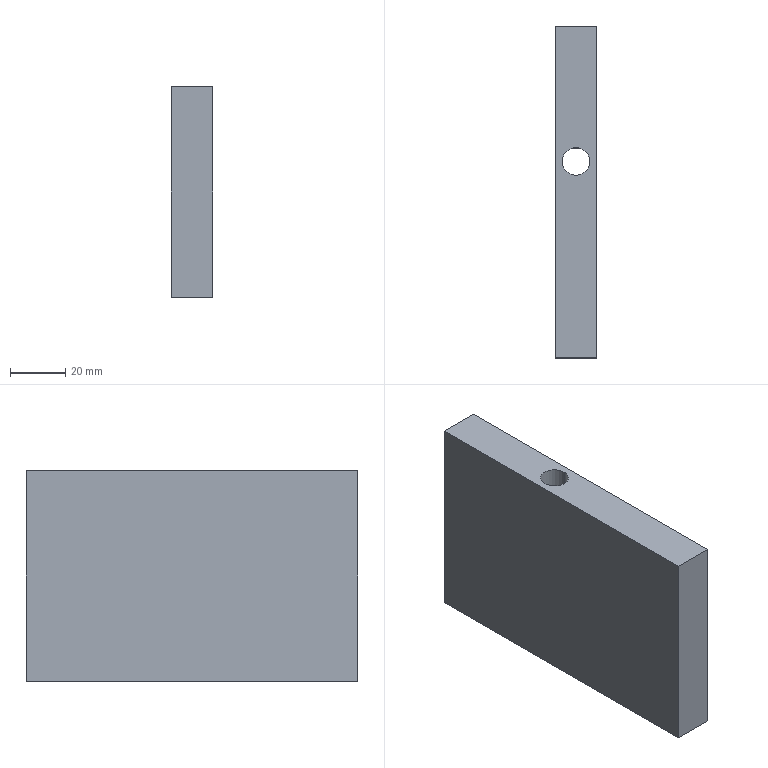Part | SolidWorks | features Extrusion 1, ICE 1 | 1 solid | 8 faces | box 15 x 120 x 76 mm | volume 130831 mm3 | plane 6 | cylinder 2 | commonest cylinder face diameters 10 x2
STEP:
#1=CARTESIAN_POINT('',(-5.,11.,0.));
#2=VERTEX_POINT('',#1);
#3=CARTESIAN_POINT('',(5.,11.,0.));
#4=VERTEX_POINT('',#3);
#5=CARTESIAN_POINT('',(0.,11.,0.));
#6=DIRECTION('',(0.,0.,1.));
#7=DIRECTION('',(1.,0.,0.));
#8=AXIS2_PLACEMENT_3D('',#5,#6,#7);
#9=CIRCLE('',#8,5.);
#10=EDGE_CURVE('',#2,#4,#9,.T.);
#11=ORIENTED_EDGE('',*,*,#10,.F.);
#12=CARTESIAN_POINT('',(-5.,11.,76.));
#13=VERTEX_POINT('',#12);
#14=CARTESIAN_POINT('',(-5.,11.,0.));
#15=DIRECTION('',(0.,0.,1.));
#16=VECTOR('',#15,1000.);
#17=LINE('',#14,#16);
#18=EDGE_CURVE('',#2,#13,#17,.T.);
#19=ORIENTED_EDGE('',*,*,#18,.T.);
#20=CARTESIAN_POINT('',(5.,11.,76.));
#21=VERTEX_POINT('',#20);
#22=CARTESIAN_POINT('',(0.,11.,76.));
#23=DIRECTION('',(0.,0.,1.));
#24=DIRECTION('',(1.,0.,0.));
#25=AXIS2_PLACEMENT_3D('',#22,#23,#24);
#26=CIRCLE('',#25,5.);
#27=EDGE_CURVE('',#13,#21,#26,.T.);
#28=ORIENTED_EDGE('',*,*,#27,.T.);
#29=CARTESIAN_POINT('',(5.,11.,0.));
#30=DIRECTION('',(0.,0.,1.));
#31=VECTOR('',#30,1000.);
#32=LINE('',#29,#31);
#33=EDGE_CURVE('',#4,#21,#32,.T.);
#34=ORIENTED_EDGE('',*,*,#33,.F.);
#35=EDGE_LOOP('',(#11,#19,#28,#34));
#36=FACE_OUTER_BOUND('',#35,.T.);
#37=CARTESIAN_POINT('',(0.,11.,0.));
#38=DIRECTION('',(0.,0.,1.));
#39=DIRECTION('',(1.,0.,0.));
#40=AXIS2_PLACEMENT_3D('',#37,#38,#39);
#41=CYLINDRICAL_SURFACE('',#40,5.);
#42=ADVANCED_FACE('',(#36),#41,.F.);
#43=CARTESIAN_POINT('',(-7.5,60.,0.));
#44=VERTEX_POINT('',#43);
#45=CARTESIAN_POINT('',(-7.5,-60.,0.));
#46=VERTEX_POINT('',#45);
#47=CARTESIAN_POINT('',(-7.5,-60.,0.));
#48=DIRECTION('',(0.,-1.,0.));
#49=VECTOR('',#48,1000.);
#50=LINE('',#47,#49);
#51=EDGE_CURVE('',#44,#46,#50,.T.);
#52=ORIENTED_EDGE('',*,*,#51,.T.);
#53=CARTESIAN_POINT('',(-7.5,-60.,76.));
#54=VERTEX_POINT('',#53);
#55=CARTESIAN_POINT('',(-7.5,-60.,76.));
#56=DIRECTION('',(0.,0.,-1.));
#57=VECTOR('',#56,1000.);
#58=LINE('',#55,#57);
#59=EDGE_CURVE('',#54,#46,#58,.T.);
#60=ORIENTED_EDGE('',*,*,#59,.F.);
#61=CARTESIAN_POINT('',(-7.5,60.,76.));
#62=VERTEX_POINT('',#61);
#63=CARTESIAN_POINT('',(-7.5,-60.,76.));
#64=DIRECTION('',(0.,-1.,0.));
#65=VECTOR('',#64,1000.);
#66=LINE('',#63,#65);
#67=EDGE_CURVE('',#62,#54,#66,.T.);
#68=ORIENTED_EDGE('',*,*,#67,.F.);
#69=CARTESIAN_POINT('',(-7.5,60.,76.));
#70=DIRECTION('',(0.,0.,-1.));
#71=VECTOR('',#70,1000.);
#72=LINE('',#69,#71);
#73=EDGE_CURVE('',#62,#44,#72,.T.);
#74=ORIENTED_EDGE('',*,*,#73,.T.);
#75=EDGE_LOOP('',(#52,#60,#68,#74));
#76=FACE_OUTER_BOUND('',#75,.T.);
#77=CARTESIAN_POINT('',(-7.5,-60.,76.));
#78=DIRECTION('',(1.,0.,0.));
#79=DIRECTION('',(0.,0.,-1.));
#80=AXIS2_PLACEMENT_3D('',#77,#78,#79);
#81=PLANE('',#80);
#82=ADVANCED_FACE('',(#76),#81,.F.);
#83=CARTESIAN_POINT('',(7.5,-60.,0.));
#84=VERTEX_POINT('',#83);
#85=CARTESIAN_POINT('',(7.5,-60.,0.));
#86=DIRECTION('',(1.,0.,0.));
#87=VECTOR('',#86,1000.);
#88=LINE('',#85,#87);
#89=EDGE_CURVE('',#46,#84,#88,.T.);
#90=ORIENTED_EDGE('',*,*,#89,.T.);
#91=CARTESIAN_POINT('',(7.5,-60.,76.));
#92=VERTEX_POINT('',#91);
#93=CARTESIAN_POINT('',(7.5,-60.,76.));
#94=DIRECTION('',(0.,0.,-1.));
#95=VECTOR('',#94,1000.);
#96=LINE('',#93,#95);
#97=EDGE_CURVE('',#92,#84,#96,.T.);
#98=ORIENTED_EDGE('',*,*,#97,.F.);
#99=CARTESIAN_POINT('',(7.5,-60.,76.));
#100=DIRECTION('',(1.,0.,0.));
#101=VECTOR('',#100,1000.);
#102=LINE('',#99,#101);
#103=EDGE_CURVE('',#54,#92,#102,.T.);
#104=ORIENTED_EDGE('',*,*,#103,.F.);
#105=ORIENTED_EDGE('',*,*,#59,.T.);
#106=EDGE_LOOP('',(#90,#98,#104,#105));
#107=FACE_OUTER_BOUND('',#106,.T.);
#108=CARTESIAN_POINT('',(7.5,-60.,76.));
#109=DIRECTION('',(0.,1.,0.));
#110=DIRECTION('',(0.,0.,1.));
#111=AXIS2_PLACEMENT_3D('',#108,#109,#110);
#112=PLANE('',#111);
#113=ADVANCED_FACE('',(#107),#112,.F.);
#114=CARTESIAN_POINT('',(7.5,60.,0.));
#115=VERTEX_POINT('',#114);
#116=CARTESIAN_POINT('',(7.5,-60.,0.));
#117=DIRECTION('',(0.,1.,0.));
#118=VECTOR('',#117,1000.);
#119=LINE('',#116,#118);
#120=EDGE_CURVE('',#84,#115,#119,.T.);
#121=ORIENTED_EDGE('',*,*,#120,.T.);
#122=CARTESIAN_POINT('',(7.5,60.,76.));
#123=VERTEX_POINT('',#122);
#124=CARTESIAN_POINT('',(7.5,60.,76.));
#125=DIRECTION('',(0.,0.,-1.));
#126=VECTOR('',#125,1000.);
#127=LINE('',#124,#126);
#128=EDGE_CURVE('',#123,#115,#127,.T.);
#129=ORIENTED_EDGE('',*,*,#128,.F.);
#130=CARTESIAN_POINT('',(7.5,-60.,76.));
#131=DIRECTION('',(0.,1.,0.));
#132=VECTOR('',#131,1000.);
#133=LINE('',#130,#132);
#134=EDGE_CURVE('',#92,#123,#133,.T.);
#135=ORIENTED_EDGE('',*,*,#134,.F.);
#136=ORIENTED_EDGE('',*,*,#97,.T.);
#137=EDGE_LOOP('',(#121,#129,#135,#136));
#138=FACE_OUTER_BOUND('',#137,.T.);
#139=CARTESIAN_POINT('',(7.5,-60.,76.));
#140=DIRECTION('',(-1.,0.,0.));
#141=DIRECTION('',(0.,0.,1.));
#142=AXIS2_PLACEMENT_3D('',#139,#140,#141);
#143=PLANE('',#142);
#144=ADVANCED_FACE('',(#138),#143,.F.);
#145=CARTESIAN_POINT('',(7.5,60.,0.));
#146=DIRECTION('',(-1.,0.,0.));
#147=VECTOR('',#146,1000.);
#148=LINE('',#145,#147);
#149=EDGE_CURVE('',#115,#44,#148,.T.);
#150=ORIENTED_EDGE('',*,*,#149,.T.);
#151=ORIENTED_EDGE('',*,*,#73,.F.);
#152=CARTESIAN_POINT('',(7.5,60.,76.));
#153=DIRECTION('',(-1.,0.,0.));
#154=VECTOR('',#153,1000.);
#155=LINE('',#152,#154);
#156=EDGE_CURVE('',#123,#62,#155,.T.);
#157=ORIENTED_EDGE('',*,*,#156,.F.);
#158=ORIENTED_EDGE('',*,*,#128,.T.);
#159=EDGE_LOOP('',(#150,#151,#157,#158));
#160=FACE_OUTER_BOUND('',#159,.T.);
#161=CARTESIAN_POINT('',(7.5,60.,76.));
#162=DIRECTION('',(0.,-1.,0.));
#163=DIRECTION('',(0.,0.,-1.));
#164=AXIS2_PLACEMENT_3D('',#161,#162,#163);
#165=PLANE('',#164);
#166=ADVANCED_FACE('',(#160),#165,.F.);
#167=CARTESIAN_POINT('',(0.,11.,76.));
#168=DIRECTION('',(0.,0.,1.));
#169=DIRECTION('',(1.,0.,0.));
#170=AXIS2_PLACEMENT_3D('',#167,#168,#169);
#171=CIRCLE('',#170,5.);
#172=EDGE_CURVE('',#21,#13,#171,.T.);
#173=ORIENTED_EDGE('',*,*,#172,.F.);
#174=ORIENTED_EDGE('',*,*,#27,.F.);
#175=EDGE_LOOP('',(#173,#174));
#176=FACE_BOUND('',#175,.T.);
#177=ORIENTED_EDGE('',*,*,#67,.T.);
#178=ORIENTED_EDGE('',*,*,#103,.T.);
#179=ORIENTED_EDGE('',*,*,#134,.T.);
#180=ORIENTED_EDGE('',*,*,#156,.T.);
#181=EDGE_LOOP('',(#177,#178,#179,#180));
#182=FACE_OUTER_BOUND('',#181,.T.);
#183=CARTESIAN_POINT('',(0.,0.,76.));
#184=DIRECTION('',(0.,0.,1.));
#185=DIRECTION('',(1.,0.,0.));
#186=AXIS2_PLACEMENT_3D('',#183,#184,#185);
#187=PLANE('',#186);
#188=ADVANCED_FACE('',(#176,#182),#187,.T.);
#189=CARTESIAN_POINT('',(0.,11.,0.));
#190=DIRECTION('',(0.,0.,1.));
#191=DIRECTION('',(1.,0.,0.));
#192=AXIS2_PLACEMENT_3D('',#189,#190,#191);
#193=CIRCLE('',#192,5.);
#194=EDGE_CURVE('',#4,#2,#193,.T.);
#195=ORIENTED_EDGE('',*,*,#194,.T.);
#196=ORIENTED_EDGE('',*,*,#10,.T.);
#197=EDGE_LOOP('',(#195,#196));
#198=FACE_BOUND('',#197,.T.);
#199=ORIENTED_EDGE('',*,*,#51,.F.);
#200=ORIENTED_EDGE('',*,*,#149,.F.);
#201=ORIENTED_EDGE('',*,*,#120,.F.);
#202=ORIENTED_EDGE('',*,*,#89,.F.);
#203=EDGE_LOOP('',(#199,#200,#201,#202));
#204=FACE_OUTER_BOUND('',#203,.T.);
#205=CARTESIAN_POINT('',(0.,0.,0.));
#206=DIRECTION('',(0.,0.,1.));
#207=DIRECTION('',(1.,0.,0.));
#208=AXIS2_PLACEMENT_3D('',#205,#206,#207);
#209=PLANE('',#208);
#210=ADVANCED_FACE('',(#198,#204),#209,.F.);
#211=ORIENTED_EDGE('',*,*,#18,.F.);
#212=ORIENTED_EDGE('',*,*,#194,.F.);
#213=ORIENTED_EDGE('',*,*,#33,.T.);
#214=ORIENTED_EDGE('',*,*,#172,.T.);
#215=EDGE_LOOP('',(#211,#212,#213,#214));
#216=FACE_OUTER_BOUND('',#215,.T.);
#217=CARTESIAN_POINT('',(0.,11.,0.));
#218=DIRECTION('',(0.,0.,1.));
#219=DIRECTION('',(1.,0.,0.));
#220=AXIS2_PLACEMENT_3D('',#217,#218,#219);
#221=CYLINDRICAL_SURFACE('',#220,5.);
#222=ADVANCED_FACE('',(#216),#221,.F.);
#223=CLOSED_SHELL('',(#42,#82,#113,#144,#166,#188,#210,#222));
#224=MANIFOLD_SOLID_BREP('',#223);
#225=CARTESIAN_POINT('',(0.,0.,0.));
#226=DIRECTION('',(0.,0.,1.));
#227=DIRECTION('',(1.,0.,0.));
#228=AXIS2_PLACEMENT_3D('',#225,#226,#227);
#229=(LENGTH_UNIT()NAMED_UNIT(*)SI_UNIT(.MILLI.,.METRE.));
#230=UNCERTAINTY_MEASURE_WITH_UNIT(LENGTH_MEASURE(0.00001),#229,'','');
#231=(NAMED_UNIT(*)PLANE_ANGLE_UNIT()SI_UNIT($,.RADIAN.));
#232=(NAMED_UNIT(*)SI_UNIT($,.STERADIAN.)SOLID_ANGLE_UNIT());
#233=(GEOMETRIC_REPRESENTATION_CONTEXT(3)GLOBAL_UNCERTAINTY_ASSIGNED_CONTEXT((#230))GLOBAL_UNIT_ASSIGNED_CONTEXT((#229,#231,#232))REPRESENTATION_CONTEXT('',''));
#234=ADVANCED_BREP_SHAPE_REPRESENTATION('',(#224,#228),#233);